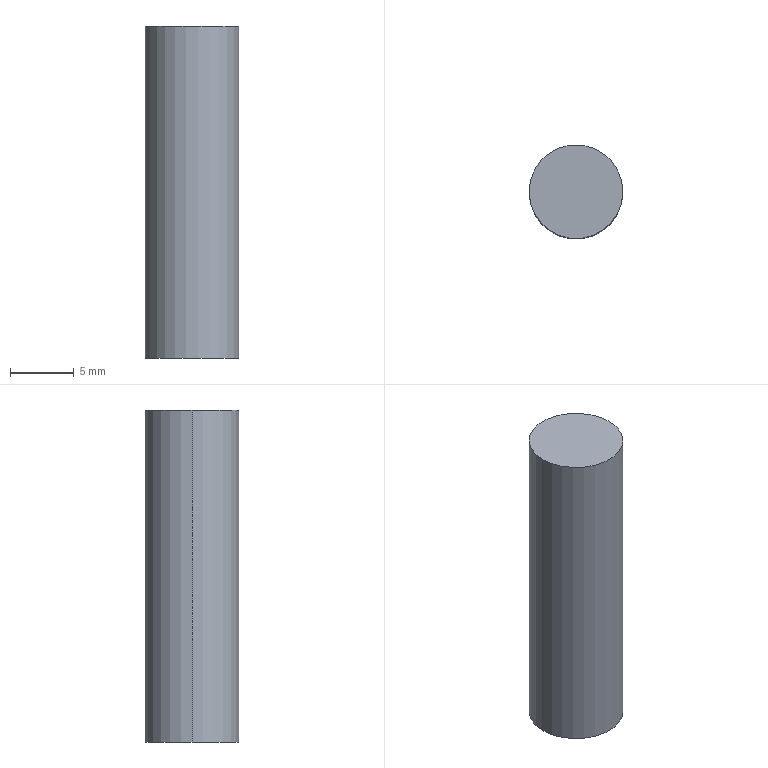Part | SolidWorks | features Extrusion 1 | 1 solid | 4 faces | box 7.349 x 7.349 x 26 mm | volume 1103 mm3 | cylinder 2 | plane 2 | commonest cylinder face diameters 7.349 x2
STEP:
#1=CARTESIAN_POINT('',(-23.391,16.289,13.));
#2=VERTEX_POINT('',#1);
#3=CARTESIAN_POINT('',(-30.74,16.289,13.));
#4=VERTEX_POINT('',#3);
#5=CARTESIAN_POINT('',(-27.066,16.289,13.));
#6=DIRECTION('',(0.,0.,1.));
#7=DIRECTION('',(1.,0.,0.));
#8=AXIS2_PLACEMENT_3D('',#5,#6,#7);
#9=CIRCLE('',#8,3.675);
#10=EDGE_CURVE('',#2,#4,#9,.T.);
#11=ORIENTED_EDGE('',*,*,#10,.F.);
#12=CARTESIAN_POINT('',(-23.391,16.289,-13.));
#13=VERTEX_POINT('',#12);
#14=CARTESIAN_POINT('',(-23.391,16.289,13.));
#15=DIRECTION('',(0.,0.,-1.));
#16=VECTOR('',#15,1000.);
#17=LINE('',#14,#16);
#18=EDGE_CURVE('',#2,#13,#17,.T.);
#19=ORIENTED_EDGE('',*,*,#18,.T.);
#20=CARTESIAN_POINT('',(-30.74,16.289,-13.));
#21=VERTEX_POINT('',#20);
#22=CARTESIAN_POINT('',(-27.066,16.289,-13.));
#23=DIRECTION('',(0.,0.,1.));
#24=DIRECTION('',(1.,0.,0.));
#25=AXIS2_PLACEMENT_3D('',#22,#23,#24);
#26=CIRCLE('',#25,3.675);
#27=EDGE_CURVE('',#13,#21,#26,.T.);
#28=ORIENTED_EDGE('',*,*,#27,.T.);
#29=CARTESIAN_POINT('',(-30.74,16.289,13.));
#30=DIRECTION('',(0.,0.,-1.));
#31=VECTOR('',#30,1000.);
#32=LINE('',#29,#31);
#33=EDGE_CURVE('',#4,#21,#32,.T.);
#34=ORIENTED_EDGE('',*,*,#33,.F.);
#35=EDGE_LOOP('',(#11,#19,#28,#34));
#36=FACE_OUTER_BOUND('',#35,.T.);
#37=CARTESIAN_POINT('',(-27.066,16.289,13.));
#38=DIRECTION('',(0.,0.,-1.));
#39=DIRECTION('',(-1.,0.,0.));
#40=AXIS2_PLACEMENT_3D('',#37,#38,#39);
#41=CYLINDRICAL_SURFACE('',#40,3.675);
#42=ADVANCED_FACE('',(#36),#41,.T.);
#43=ORIENTED_EDGE('',*,*,#18,.F.);
#44=CARTESIAN_POINT('',(-27.066,16.289,13.));
#45=DIRECTION('',(0.,0.,1.));
#46=DIRECTION('',(1.,0.,0.));
#47=AXIS2_PLACEMENT_3D('',#44,#45,#46);
#48=CIRCLE('',#47,3.675);
#49=EDGE_CURVE('',#4,#2,#48,.T.);
#50=ORIENTED_EDGE('',*,*,#49,.F.);
#51=ORIENTED_EDGE('',*,*,#33,.T.);
#52=CARTESIAN_POINT('',(-27.066,16.289,-13.));
#53=DIRECTION('',(0.,0.,1.));
#54=DIRECTION('',(1.,0.,0.));
#55=AXIS2_PLACEMENT_3D('',#52,#53,#54);
#56=CIRCLE('',#55,3.675);
#57=EDGE_CURVE('',#21,#13,#56,.T.);
#58=ORIENTED_EDGE('',*,*,#57,.T.);
#59=EDGE_LOOP('',(#43,#50,#51,#58));
#60=FACE_OUTER_BOUND('',#59,.T.);
#61=CARTESIAN_POINT('',(-27.066,16.289,13.));
#62=DIRECTION('',(0.,0.,-1.));
#63=DIRECTION('',(-1.,0.,0.));
#64=AXIS2_PLACEMENT_3D('',#61,#62,#63);
#65=CYLINDRICAL_SURFACE('',#64,3.675);
#66=ADVANCED_FACE('',(#60),#65,.T.);
#67=ORIENTED_EDGE('',*,*,#49,.T.);
#68=ORIENTED_EDGE('',*,*,#10,.T.);
#69=EDGE_LOOP('',(#67,#68));
#70=FACE_OUTER_BOUND('',#69,.T.);
#71=CARTESIAN_POINT('',(-27.066,16.289,13.));
#72=DIRECTION('',(0.,0.,1.));
#73=DIRECTION('',(1.,0.,0.));
#74=AXIS2_PLACEMENT_3D('',#71,#72,#73);
#75=PLANE('',#74);
#76=ADVANCED_FACE('',(#70),#75,.T.);
#77=ORIENTED_EDGE('',*,*,#57,.F.);
#78=ORIENTED_EDGE('',*,*,#27,.F.);
#79=EDGE_LOOP('',(#77,#78));
#80=FACE_OUTER_BOUND('',#79,.T.);
#81=CARTESIAN_POINT('',(-27.066,16.289,-13.));
#82=DIRECTION('',(0.,0.,1.));
#83=DIRECTION('',(1.,0.,0.));
#84=AXIS2_PLACEMENT_3D('',#81,#82,#83);
#85=PLANE('',#84);
#86=ADVANCED_FACE('',(#80),#85,.F.);
#87=CLOSED_SHELL('',(#42,#66,#76,#86));
#88=MANIFOLD_SOLID_BREP('',#87);
#89=CARTESIAN_POINT('',(0.,0.,0.));
#90=DIRECTION('',(0.,0.,1.));
#91=DIRECTION('',(1.,0.,0.));
#92=AXIS2_PLACEMENT_3D('',#89,#90,#91);
#93=(LENGTH_UNIT()NAMED_UNIT(*)SI_UNIT(.MILLI.,.METRE.));
#94=UNCERTAINTY_MEASURE_WITH_UNIT(LENGTH_MEASURE(0.00001),#93,'','');
#95=(NAMED_UNIT(*)PLANE_ANGLE_UNIT()SI_UNIT($,.RADIAN.));
#96=(NAMED_UNIT(*)SI_UNIT($,.STERADIAN.)SOLID_ANGLE_UNIT());
#97=(GEOMETRIC_REPRESENTATION_CONTEXT(3)GLOBAL_UNCERTAINTY_ASSIGNED_CONTEXT((#94))GLOBAL_UNIT_ASSIGNED_CONTEXT((#93,#95,#96))REPRESENTATION_CONTEXT('',''));
#98=ADVANCED_BREP_SHAPE_REPRESENTATION('',(#88,#92),#97);